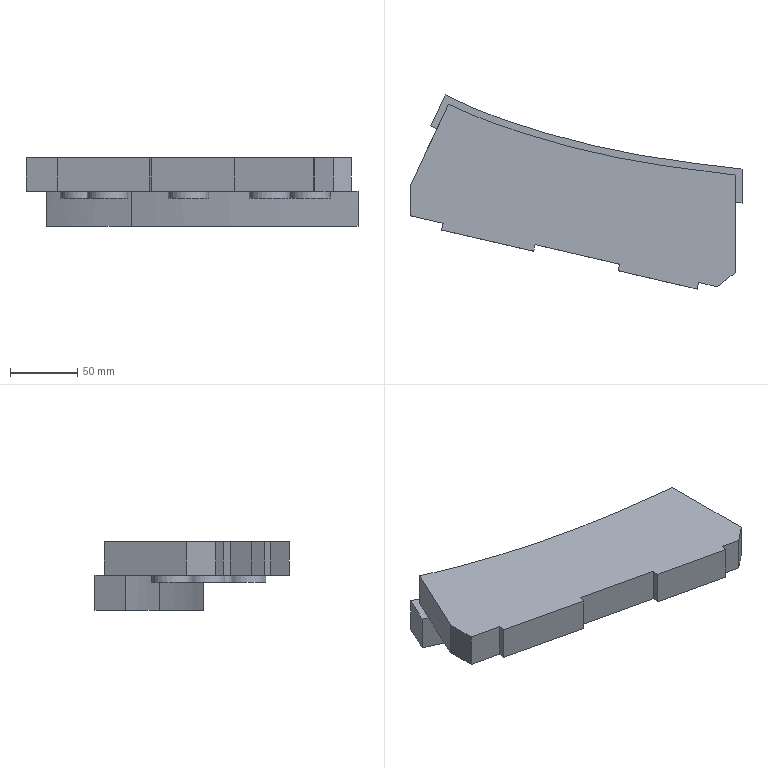Part | NX | features solid 2 | 1 solid | 35 faces | box 246.107 x 143.832 x 51 mm | volume 655442 mm3 | plane 25 | spline 5 | cylinder 5 | commonest cylinder face diameters 30 x5
STEP:
#1=CARTESIAN_POINT('',(-485.611,-295.558,20.));
#2=VERTEX_POINT('',#1);
#3=CARTESIAN_POINT('',(-470.611,-295.558,20.));
#4=DIRECTION('',(0.,0.,-1.));
#5=DIRECTION('',(-1.,0.,0.));
#6=AXIS2_PLACEMENT_3D('',#3,#4,#5);
#7=CIRCLE('',#6,15.);
#8=EDGE_CURVE('',#2,#2,#7,.T.);
#9=ORIENTED_EDGE('',*,*,#8,.F.);
#10=EDGE_LOOP('',(#9));
#11=FACE_BOUND('',#10,.T.);
#12=CARTESIAN_POINT('',(-625.611,-240.558,20.));
#13=VERTEX_POINT('',#12);
#14=CARTESIAN_POINT('',(-610.611,-240.558,20.));
#15=DIRECTION('',(0.,0.,-1.));
#16=DIRECTION('',(-1.,0.,0.));
#17=AXIS2_PLACEMENT_3D('',#14,#15,#16);
#18=CIRCLE('',#17,15.);
#19=EDGE_CURVE('',#13,#13,#18,.T.);
#20=ORIENTED_EDGE('',*,*,#19,.F.);
#21=EDGE_LOOP('',(#20));
#22=FACE_BOUND('',#21,.T.);
#23=CARTESIAN_POINT('',(-410.,-315.453,20.));
#24=VERTEX_POINT('',#23);
#25=CARTESIAN_POINT('',(-410.,-263.355,20.));
#26=VERTEX_POINT('',#25);
#27=CARTESIAN_POINT('',(-410.,-330.218,20.));
#28=DIRECTION('',(0.,-1.,0.));
#29=VECTOR('',#28,1000.);
#30=LINE('',#27,#29);
#31=EDGE_CURVE('',#24,#26,#30,.F.);
#32=ORIENTED_EDGE('',*,*,#31,.F.);
#33=CARTESIAN_POINT('',(-423.262,-326.002,20.));
#34=VERTEX_POINT('',#33);
#35=CARTESIAN_POINT('',(-426.375,-328.478,20.));
#36=DIRECTION('',(-0.7826,-0.6225,0.));
#37=VECTOR('',#36,1000.);
#38=LINE('',#35,#37);
#39=EDGE_CURVE('',#24,#34,#38,.T.);
#40=ORIENTED_EDGE('',*,*,#39,.T.);
#41=CARTESIAN_POINT('',(-437.198,-322.785,20.));
#42=VERTEX_POINT('',#41);
#43=CARTESIAN_POINT('',(-647.681,-274.191,20.));
#44=DIRECTION('',(-0.9744,0.225,0.));
#45=VECTOR('',#44,1000.);
#46=LINE('',#43,#45);
#47=EDGE_CURVE('',#42,#34,#46,.F.);
#48=ORIENTED_EDGE('',*,*,#47,.F.);
#49=CARTESIAN_POINT('',(-438.323,-327.657,20.));
#50=VERTEX_POINT('',#49);
#51=CARTESIAN_POINT('',(-418.412,-241.415,20.));
#52=DIRECTION('',(0.225,0.9744,0.));
#53=VECTOR('',#52,1000.);
#54=LINE('',#51,#53);
#55=EDGE_CURVE('',#42,#50,#54,.F.);
#56=ORIENTED_EDGE('',*,*,#55,.T.);
#57=CARTESIAN_POINT('',(-496.785,-314.16,20.));
#58=VERTEX_POINT('',#57);
#59=CARTESIAN_POINT('',(-360.373,-345.653,20.));
#60=DIRECTION('',(0.9744,-0.225,0.));
#61=VECTOR('',#60,1000.);
#62=LINE('',#59,#61);
#63=EDGE_CURVE('',#58,#50,#62,.T.);
#64=ORIENTED_EDGE('',*,*,#63,.F.);
#65=CARTESIAN_POINT('',(-495.66,-309.288,20.));
#66=VERTEX_POINT('',#65);
#67=CARTESIAN_POINT('',(-476.874,-227.918,20.));
#68=DIRECTION('',(0.225,0.9744,0.));
#69=VECTOR('',#68,1000.);
#70=LINE('',#67,#69);
#71=EDGE_CURVE('',#66,#58,#70,.F.);
#72=ORIENTED_EDGE('',*,*,#71,.F.);
#73=CARTESIAN_POINT('',(-558.405,-294.802,20.));
#74=VERTEX_POINT('',#73);
#75=CARTESIAN_POINT('',(-647.681,-274.191,20.));
#76=DIRECTION('',(-0.9744,0.225,0.));
#77=VECTOR('',#76,1000.);
#78=LINE('',#75,#77);
#79=EDGE_CURVE('',#74,#66,#78,.F.);
#80=ORIENTED_EDGE('',*,*,#79,.F.);
#81=CARTESIAN_POINT('',(-559.529,-299.674,20.));
#82=VERTEX_POINT('',#81);
#83=CARTESIAN_POINT('',(-539.619,-213.432,20.));
#84=DIRECTION('',(0.225,0.9744,0.));
#85=VECTOR('',#84,1000.);
#86=LINE('',#83,#85);
#87=EDGE_CURVE('',#74,#82,#86,.F.);
#88=ORIENTED_EDGE('',*,*,#87,.T.);
#89=CARTESIAN_POINT('',(-627.735,-283.927,20.));
#90=VERTEX_POINT('',#89);
#91=CARTESIAN_POINT('',(-598.504,-290.676,20.));
#92=DIRECTION('',(0.9744,-0.225,0.));
#93=VECTOR('',#92,1000.);
#94=LINE('',#91,#93);
#95=EDGE_CURVE('',#90,#82,#94,.T.);
#96=ORIENTED_EDGE('',*,*,#95,.F.);
#97=CARTESIAN_POINT('',(-626.611,-279.056,20.));
#98=VERTEX_POINT('',#97);
#99=CARTESIAN_POINT('',(-607.825,-197.685,20.));
#100=DIRECTION('',(0.225,0.9744,0.));
#101=VECTOR('',#100,1000.);
#102=LINE('',#99,#101);
#103=EDGE_CURVE('',#98,#90,#102,.F.);
#104=ORIENTED_EDGE('',*,*,#103,.F.);
#105=CARTESIAN_POINT('',(-651.107,-273.4,20.));
#106=VERTEX_POINT('',#105);
#107=CARTESIAN_POINT('',(-647.681,-274.191,20.));
#108=DIRECTION('',(-0.9744,0.225,0.));
#109=VECTOR('',#108,1000.);
#110=LINE('',#107,#109);
#111=EDGE_CURVE('',#106,#98,#110,.F.);
#112=ORIENTED_EDGE('',*,*,#111,.F.);
#113=CARTESIAN_POINT('',(-651.107,-251.643,20.));
#114=VERTEX_POINT('',#113);
#115=CARTESIAN_POINT('',(-651.107,-207.42,20.));
#116=DIRECTION('',(0.,1.,0.));
#117=VECTOR('',#116,1000.);
#118=LINE('',#115,#117);
#119=EDGE_CURVE('',#114,#106,#118,.F.);
#120=ORIENTED_EDGE('',*,*,#119,.F.);
#121=CARTESIAN_POINT('',(-631.107,-208.753,20.));
#122=VERTEX_POINT('',#121);
#123=CARTESIAN_POINT('',(-622.584,-190.474,20.));
#124=DIRECTION('',(0.4226,0.9063,0.));
#125=VECTOR('',#124,1000.);
#126=LINE('',#123,#125);
#127=EDGE_CURVE('',#122,#114,#126,.F.);
#128=ORIENTED_EDGE('',*,*,#127,.F.);
#129=CARTESIAN_POINT('',(-572.969,-231.328,20.));
#130=VERTEX_POINT('',#129);
#131=CARTESIAN_POINT('',(-572.969,-231.328,20.));
#132=CARTESIAN_POINT('',(-592.888,-225.076,20.));
#133=CARTESIAN_POINT('',(-612.439,-217.955,20.));
#134=CARTESIAN_POINT('',(-631.107,-208.753,20.));
#135=B_SPLINE_CURVE_WITH_KNOTS('',3,(#131,#132,#133,#134),.UNSPECIFIED.,.F.,.F.,(4,4),(0.5429,0.6055),.UNSPECIFIED.);
#136=EDGE_CURVE('',#130,#122,#135,.T.);
#137=ORIENTED_EDGE('',*,*,#136,.F.);
#138=CARTESIAN_POINT('',(-572.969,-231.328,20.));
#139=VERTEX_POINT('',#138);
#140=CARTESIAN_POINT('',(-600.393,-321.029,20.));
#141=DIRECTION('',(-0.2924,-0.9563,0.));
#142=VECTOR('',#141,1000.);
#143=LINE('',#140,#142);
#144=EDGE_CURVE('',#130,#139,#143,.F.);
#145=ORIENTED_EDGE('',*,*,#144,.T.);
#146=CARTESIAN_POINT('',(-410.,-263.355,20.));
#147=CARTESIAN_POINT('',(-423.782,-261.77,20.));
#148=CARTESIAN_POINT('',(-451.325,-258.441,20.));
#149=CARTESIAN_POINT('',(-492.449,-252.102,20.));
#150=CARTESIAN_POINT('',(-533.139,-243.268,20.));
#151=CARTESIAN_POINT('',(-559.734,-235.479,20.));
#152=CARTESIAN_POINT('',(-572.969,-231.328,20.));
#153=B_SPLINE_CURVE_WITH_KNOTS('',3,(#146,#147,#148,#149,#150,#151,#152),.UNSPECIFIED.,.F.,.F.,(4,1,1,1,4),(1.31,1.352,1.393,1.435,1.476),.UNSPECIFIED.);
#154=EDGE_CURVE('',#26,#139,#153,.T.);
#155=ORIENTED_EDGE('',*,*,#154,.F.);
#156=EDGE_LOOP('',(#32,#40,#48,#56,#64,#72,#80,#88,#96,#104,#112,#120,#128,#137,#145,#155));
#157=FACE_BOUND('',#156,.T.);
#158=CARTESIAN_POINT('',(-605.611,-265.558,20.));
#159=VERTEX_POINT('',#158);
#160=CARTESIAN_POINT('',(-590.611,-265.558,20.));
#161=DIRECTION('',(0.,0.,-1.));
#162=DIRECTION('',(-1.,0.,0.));
#163=AXIS2_PLACEMENT_3D('',#160,#161,#162);
#164=CIRCLE('',#163,15.);
#165=EDGE_CURVE('',#159,#159,#164,.T.);
#166=ORIENTED_EDGE('',*,*,#165,.F.);
#167=EDGE_LOOP('',(#166));
#168=FACE_BOUND('',#167,.T.);
#169=CARTESIAN_POINT('',(-455.611,-280.558,20.));
#170=VERTEX_POINT('',#169);
#171=CARTESIAN_POINT('',(-440.611,-280.558,20.));
#172=DIRECTION('',(0.,0.,-1.));
#173=DIRECTION('',(-1.,0.,0.));
#174=AXIS2_PLACEMENT_3D('',#171,#172,#173);
#175=CIRCLE('',#174,15.);
#176=EDGE_CURVE('',#170,#170,#175,.T.);
#177=ORIENTED_EDGE('',*,*,#176,.F.);
#178=EDGE_LOOP('',(#177));
#179=FACE_BOUND('',#178,.T.);
#180=CARTESIAN_POINT('',(-545.611,-270.558,20.));
#181=VERTEX_POINT('',#180);
#182=CARTESIAN_POINT('',(-530.611,-270.558,20.));
#183=DIRECTION('',(0.,0.,-1.));
#184=DIRECTION('',(-1.,0.,0.));
#185=AXIS2_PLACEMENT_3D('',#182,#183,#184);
#186=CIRCLE('',#185,15.);
#187=EDGE_CURVE('',#181,#181,#186,.T.);
#188=ORIENTED_EDGE('',*,*,#187,.F.);
#189=EDGE_LOOP('',(#188));
#190=FACE_BOUND('',#189,.T.);
#191=CARTESIAN_POINT('',(-565.659,-207.42,20.));
#192=DIRECTION('',(0.,0.,-1.));
#193=DIRECTION('',(-1.,0.,0.));
#194=AXIS2_PLACEMENT_3D('',#191,#192,#193);
#195=PLANE('',#194);
#196=ADVANCED_FACE('',(#11,#22,#157,#168,#179,#190),#195,.T.);
#197=CARTESIAN_POINT('',(-437.198,-322.785,45.));
#198=VERTEX_POINT('',#197);
#199=CARTESIAN_POINT('',(-423.262,-326.002,45.));
#200=VERTEX_POINT('',#199);
#201=CARTESIAN_POINT('',(-647.681,-274.191,45.));
#202=DIRECTION('',(0.9744,-0.225,0.));
#203=VECTOR('',#202,1000.);
#204=LINE('',#201,#203);
#205=EDGE_CURVE('',#198,#200,#204,.T.);
#206=ORIENTED_EDGE('',*,*,#205,.T.);
#207=CARTESIAN_POINT('',(-410.,-315.453,45.));
#208=VERTEX_POINT('',#207);
#209=CARTESIAN_POINT('',(-891.318,-698.311,45.));
#210=DIRECTION('',(-0.7826,-0.6225,0.));
#211=VECTOR('',#210,1000.);
#212=LINE('',#209,#211);
#213=EDGE_CURVE('',#200,#208,#212,.F.);
#214=ORIENTED_EDGE('',*,*,#213,.T.);
#215=CARTESIAN_POINT('',(-410.,-243.222,45.));
#216=VERTEX_POINT('',#215);
#217=CARTESIAN_POINT('',(-410.,-330.218,45.));
#218=DIRECTION('',(0.,1.,0.));
#219=VECTOR('',#218,1000.);
#220=LINE('',#217,#219);
#221=EDGE_CURVE('',#208,#216,#220,.T.);
#222=ORIENTED_EDGE('',*,*,#221,.T.);
#223=CARTESIAN_POINT('',(-567.121,-212.202,45.));
#224=VERTEX_POINT('',#223);
#225=CARTESIAN_POINT('',(-410.,-243.222,45.));
#226=CARTESIAN_POINT('',(-423.299,-241.685,45.));
#227=CARTESIAN_POINT('',(-449.879,-238.442,45.));
#228=CARTESIAN_POINT('',(-489.484,-232.294,45.));
#229=CARTESIAN_POINT('',(-528.605,-223.762,45.));
#230=CARTESIAN_POINT('',(-554.325,-216.217,45.));
#231=CARTESIAN_POINT('',(-567.121,-212.202,45.));
#232=B_SPLINE_CURVE_WITH_KNOTS('',3,(#225,#226,#227,#228,#229,#230,#231),.UNSPECIFIED.,.F.,.F.,(4,1,1,1,4),(0.1347,0.1748,0.2149,0.2551,0.2952),.UNSPECIFIED.);
#233=EDGE_CURVE('',#216,#224,#232,.T.);
#234=ORIENTED_EDGE('',*,*,#233,.T.);
#235=CARTESIAN_POINT('',(-622.653,-190.623,45.));
#236=VERTEX_POINT('',#235);
#237=CARTESIAN_POINT('',(-567.121,-212.202,45.));
#238=CARTESIAN_POINT('',(-586.224,-206.206,45.));
#239=CARTESIAN_POINT('',(-604.924,-199.397,45.));
#240=CARTESIAN_POINT('',(-622.653,-190.623,45.));
#241=B_SPLINE_CURVE_WITH_KNOTS('',3,(#237,#238,#239,#240),.UNSPECIFIED.,.F.,.F.,(4,4),(0.,0.05934),.UNSPECIFIED.);
#242=EDGE_CURVE('',#224,#236,#241,.T.);
#243=ORIENTED_EDGE('',*,*,#242,.T.);
#244=CARTESIAN_POINT('',(-651.107,-251.643,45.));
#245=VERTEX_POINT('',#244);
#246=CARTESIAN_POINT('',(-622.584,-190.474,45.));
#247=DIRECTION('',(0.4226,0.9063,0.));
#248=VECTOR('',#247,1000.);
#249=LINE('',#246,#248);
#250=EDGE_CURVE('',#236,#245,#249,.F.);
#251=ORIENTED_EDGE('',*,*,#250,.T.);
#252=CARTESIAN_POINT('',(-651.107,-273.4,45.));
#253=VERTEX_POINT('',#252);
#254=CARTESIAN_POINT('',(-651.107,-664.302,45.));
#255=DIRECTION('',(0.,-1.,0.));
#256=VECTOR('',#255,1000.);
#257=LINE('',#254,#256);
#258=EDGE_CURVE('',#245,#253,#257,.T.);
#259=ORIENTED_EDGE('',*,*,#258,.T.);
#260=CARTESIAN_POINT('',(-626.611,-279.056,45.));
#261=VERTEX_POINT('',#260);
#262=CARTESIAN_POINT('',(-647.681,-274.191,45.));
#263=DIRECTION('',(0.9744,-0.225,0.));
#264=VECTOR('',#263,1000.);
#265=LINE('',#262,#264);
#266=EDGE_CURVE('',#253,#261,#265,.T.);
#267=ORIENTED_EDGE('',*,*,#266,.T.);
#268=CARTESIAN_POINT('',(-627.735,-283.927,45.));
#269=VERTEX_POINT('',#268);
#270=CARTESIAN_POINT('',(-725.815,-708.757,45.));
#271=DIRECTION('',(-0.225,-0.9744,0.));
#272=VECTOR('',#271,1000.);
#273=LINE('',#270,#272);
#274=EDGE_CURVE('',#261,#269,#273,.T.);
#275=ORIENTED_EDGE('',*,*,#274,.T.);
#276=CARTESIAN_POINT('',(-559.529,-299.674,45.));
#277=VERTEX_POINT('',#276);
#278=CARTESIAN_POINT('',(-598.504,-290.676,45.));
#279=DIRECTION('',(0.9744,-0.225,0.));
#280=VECTOR('',#279,1000.);
#281=LINE('',#278,#280);
#282=EDGE_CURVE('',#269,#277,#281,.T.);
#283=ORIENTED_EDGE('',*,*,#282,.T.);
#284=CARTESIAN_POINT('',(-558.405,-294.802,45.));
#285=VERTEX_POINT('',#284);
#286=CARTESIAN_POINT('',(-657.609,-724.504,45.));
#287=DIRECTION('',(-0.225,-0.9744,0.));
#288=VECTOR('',#287,1000.);
#289=LINE('',#286,#288);
#290=EDGE_CURVE('',#285,#277,#289,.T.);
#291=ORIENTED_EDGE('',*,*,#290,.F.);
#292=CARTESIAN_POINT('',(-495.66,-309.288,45.));
#293=VERTEX_POINT('',#292);
#294=CARTESIAN_POINT('',(-647.681,-274.191,45.));
#295=DIRECTION('',(0.9744,-0.225,0.));
#296=VECTOR('',#295,1000.);
#297=LINE('',#294,#296);
#298=EDGE_CURVE('',#285,#293,#297,.T.);
#299=ORIENTED_EDGE('',*,*,#298,.T.);
#300=CARTESIAN_POINT('',(-496.785,-314.16,45.));
#301=VERTEX_POINT('',#300);
#302=CARTESIAN_POINT('',(-594.865,-738.989,45.));
#303=DIRECTION('',(-0.225,-0.9744,0.));
#304=VECTOR('',#303,1000.);
#305=LINE('',#302,#304);
#306=EDGE_CURVE('',#293,#301,#305,.T.);
#307=ORIENTED_EDGE('',*,*,#306,.T.);
#308=CARTESIAN_POINT('',(-438.323,-327.657,45.));
#309=VERTEX_POINT('',#308);
#310=CARTESIAN_POINT('',(-360.373,-345.653,45.));
#311=DIRECTION('',(0.9744,-0.225,0.));
#312=VECTOR('',#311,1000.);
#313=LINE('',#310,#312);
#314=EDGE_CURVE('',#301,#309,#313,.T.);
#315=ORIENTED_EDGE('',*,*,#314,.T.);
#316=CARTESIAN_POINT('',(-536.402,-752.486,45.));
#317=DIRECTION('',(-0.225,-0.9744,0.));
#318=VECTOR('',#317,1000.);
#319=LINE('',#316,#318);
#320=EDGE_CURVE('',#198,#309,#319,.T.);
#321=ORIENTED_EDGE('',*,*,#320,.F.);
#322=EDGE_LOOP('',(#206,#214,#222,#234,#243,#251,#259,#267,#275,#283,#291,#299,#307,#315,#321));
#323=FACE_BOUND('',#322,.T.);
#324=CARTESIAN_POINT('',(-918.37,-664.302,45.));
#325=DIRECTION('',(0.,0.,1.));
#326=DIRECTION('',(1.,0.,0.));
#327=AXIS2_PLACEMENT_3D('',#324,#325,#326);
#328=PLANE('',#327);
#329=ADVANCED_FACE('',(#323),#328,.T.);
#330=CARTESIAN_POINT('',(-651.107,-273.4,70.));
#331=DIRECTION('',(0.,0.,1.));
#332=VECTOR('',#331,1000.);
#333=LINE('',#330,#332);
#334=EDGE_CURVE('',#106,#253,#333,.T.);
#335=ORIENTED_EDGE('',*,*,#334,.F.);
#336=ORIENTED_EDGE('',*,*,#111,.T.);
#337=CARTESIAN_POINT('',(-626.611,-279.056,45.));
#338=DIRECTION('',(0.,0.,-1.));
#339=VECTOR('',#338,1000.);
#340=LINE('',#337,#339);
#341=EDGE_CURVE('',#261,#98,#340,.T.);
#342=ORIENTED_EDGE('',*,*,#341,.F.);
#343=ORIENTED_EDGE('',*,*,#266,.F.);
#344=EDGE_LOOP('',(#335,#336,#342,#343));
#345=FACE_BOUND('',#344,.T.);
#346=CARTESIAN_POINT('',(-647.681,-274.191,70.));
#347=DIRECTION('',(0.225,0.9744,0.));
#348=DIRECTION('',(-0.9744,0.225,0.));
#349=AXIS2_PLACEMENT_3D('',#346,#347,#348);
#350=PLANE('',#349);
#351=ADVANCED_FACE('',(#345),#350,.F.);
#352=CARTESIAN_POINT('',(-651.107,-251.643,45.));
#353=DIRECTION('',(0.,0.,-1.));
#354=VECTOR('',#353,1000.);
#355=LINE('',#352,#354);
#356=EDGE_CURVE('',#245,#114,#355,.T.);
#357=ORIENTED_EDGE('',*,*,#356,.F.);
#358=ORIENTED_EDGE('',*,*,#250,.F.);
#359=CARTESIAN_POINT('',(-622.653,-190.623,20.));
#360=VERTEX_POINT('',#359);
#361=CARTESIAN_POINT('',(-622.653,-190.623,32.5));
#362=DIRECTION('',(0.,0.,-1.));
#363=VECTOR('',#362,1000.);
#364=LINE('',#361,#363);
#365=EDGE_CURVE('',#360,#236,#364,.F.);
#366=ORIENTED_EDGE('',*,*,#365,.F.);
#367=CARTESIAN_POINT('',(-622.584,-190.474,20.));
#368=DIRECTION('',(0.4226,0.9063,0.));
#369=VECTOR('',#368,1000.);
#370=LINE('',#367,#369);
#371=EDGE_CURVE('',#360,#122,#370,.F.);
#372=ORIENTED_EDGE('',*,*,#371,.T.);
#373=ORIENTED_EDGE('',*,*,#127,.T.);
#374=EDGE_LOOP('',(#357,#358,#366,#372,#373));
#375=FACE_BOUND('',#374,.T.);
#376=CARTESIAN_POINT('',(-622.584,-190.474,45.));
#377=DIRECTION('',(0.9063,-0.4226,0.));
#378=DIRECTION('',(0.4226,0.9063,0.));
#379=AXIS2_PLACEMENT_3D('',#376,#377,#378);
#380=PLANE('',#379);
#381=ADVANCED_FACE('',(#375),#380,.F.);
#382=CARTESIAN_POINT('',(-625.,-183.825,-6.));
#383=VERTEX_POINT('',#382);
#384=CARTESIAN_POINT('',(-635.575,-206.502,-6.));
#385=VERTEX_POINT('',#384);
#386=CARTESIAN_POINT('',(-861.431,-690.853,-6.));
#387=DIRECTION('',(-0.4226,-0.9063,0.));
#388=VECTOR('',#387,1000.);
#389=LINE('',#386,#388);
#390=EDGE_CURVE('',#383,#385,#389,.T.);
#391=ORIENTED_EDGE('',*,*,#390,.F.);
#392=CARTESIAN_POINT('',(-405.,-238.764,-6.));
#393=VERTEX_POINT('',#392);
#394=CARTESIAN_POINT('',(-625.,-183.825,-6.));
#395=CARTESIAN_POINT('',(-616.501,-188.248,-6.));
#396=CARTESIAN_POINT('',(-599.149,-196.032,-6.));
#397=CARTESIAN_POINT('',(-572.385,-205.497,-6.));
#398=CARTESIAN_POINT('',(-545.206,-213.724,-6.));
#399=CARTESIAN_POINT('',(-517.745,-221.08,-6.));
#400=CARTESIAN_POINT('',(-489.761,-226.95,-6.));
#401=CARTESIAN_POINT('',(-452.233,-233.165,-6.));
#402=CARTESIAN_POINT('',(-423.904,-236.602,-6.));
#403=CARTESIAN_POINT('',(-405.,-238.764,-6.));
#404=B_SPLINE_CURVE_WITH_KNOTS('',3,(#394,#395,#396,#397,#398,#399,#400,#401,#402,#403),.UNSPECIFIED.,.F.,.F.,(4,1,1,1,1,1,1,4),(1.776,1.803,1.83,1.857,1.884,1.911,1.938,1.992),.UNSPECIFIED.);
#405=EDGE_CURVE('',#393,#383,#404,.F.);
#406=ORIENTED_EDGE('',*,*,#405,.F.);
#407=CARTESIAN_POINT('',(-405.,-263.926,-6.));
#408=VERTEX_POINT('',#407);
#409=CARTESIAN_POINT('',(-405.,-1052.635,-6.));
#410=DIRECTION('',(0.,1.,0.));
#411=VECTOR('',#410,1000.);
#412=LINE('',#409,#411);
#413=EDGE_CURVE('',#408,#393,#412,.T.);
#414=ORIENTED_EDGE('',*,*,#413,.F.);
#415=CARTESIAN_POINT('',(-572.969,-231.328,-6.));
#416=VERTEX_POINT('',#415);
#417=CARTESIAN_POINT('',(-405.,-263.926,-6.));
#418=CARTESIAN_POINT('',(-419.214,-262.309,-6.));
#419=CARTESIAN_POINT('',(-447.641,-258.943,-6.));
#420=CARTESIAN_POINT('',(-490.009,-252.558,-6.));
#421=CARTESIAN_POINT('',(-531.843,-243.634,-6.));
#422=CARTESIAN_POINT('',(-559.299,-235.615,-6.));
#423=CARTESIAN_POINT('',(-572.969,-231.328,-6.));
#424=B_SPLINE_CURVE_WITH_KNOTS('',3,(#417,#418,#419,#420,#421,#422,#423),.UNSPECIFIED.,.F.,.F.,(4,1,1,1,4),(0.1254,0.1683,0.2112,0.2541,0.297),.UNSPECIFIED.);
#425=EDGE_CURVE('',#408,#416,#424,.T.);
#426=ORIENTED_EDGE('',*,*,#425,.T.);
#427=CARTESIAN_POINT('',(-572.969,-231.328,-6.));
#428=VERTEX_POINT('',#427);
#429=CARTESIAN_POINT('',(-971.893,-1536.153,-6.));
#430=DIRECTION('',(0.2924,0.9563,0.));
#431=VECTOR('',#430,1000.);
#432=LINE('',#429,#431);
#433=EDGE_CURVE('',#428,#416,#432,.T.);
#434=ORIENTED_EDGE('',*,*,#433,.F.);
#435=CARTESIAN_POINT('',(-572.969,-231.328,-6.));
#436=CARTESIAN_POINT('',(-594.513,-224.566,-6.));
#437=CARTESIAN_POINT('',(-615.605,-216.793,-6.));
#438=CARTESIAN_POINT('',(-635.575,-206.502,-6.));
#439=B_SPLINE_CURVE_WITH_KNOTS('',3,(#435,#436,#437,#438),.UNSPECIFIED.,.F.,.F.,(4,4),(0.,0.06729),.UNSPECIFIED.);
#440=EDGE_CURVE('',#428,#385,#439,.T.);
#441=ORIENTED_EDGE('',*,*,#440,.T.);
#442=EDGE_LOOP('',(#391,#406,#414,#426,#434,#441));
#443=FACE_BOUND('',#442,.T.);
#444=CARTESIAN_POINT('',(-918.37,-664.302,-6.));
#445=DIRECTION('',(0.,0.,1.));
#446=DIRECTION('',(1.,0.,0.));
#447=AXIS2_PLACEMENT_3D('',#444,#445,#446);
#448=PLANE('',#447);
#449=ADVANCED_FACE('',(#443),#448,.F.);
#450=CARTESIAN_POINT('',(-625.,-183.825,20.));
#451=VERTEX_POINT('',#450);
#452=CARTESIAN_POINT('',(-625.,-183.825,7.));
#453=DIRECTION('',(0.,0.,-1.));
#454=VECTOR('',#453,1000.);
#455=LINE('',#452,#454);
#456=EDGE_CURVE('',#451,#383,#455,.T.);
#457=ORIENTED_EDGE('',*,*,#456,.F.);
#458=CARTESIAN_POINT('',(-405.,-238.764,20.));
#459=VERTEX_POINT('',#458);
#460=CARTESIAN_POINT('',(-625.,-183.825,20.));
#461=CARTESIAN_POINT('',(-616.51,-188.243,20.));
#462=CARTESIAN_POINT('',(-599.168,-196.025,20.));
#463=CARTESIAN_POINT('',(-572.395,-205.494,20.));
#464=CARTESIAN_POINT('',(-545.198,-213.727,20.));
#465=CARTESIAN_POINT('',(-517.694,-221.092,20.));
#466=CARTESIAN_POINT('',(-489.704,-226.961,20.));
#467=CARTESIAN_POINT('',(-452.21,-233.167,20.));
#468=CARTESIAN_POINT('',(-423.894,-236.603,20.));
#469=CARTESIAN_POINT('',(-405.,-238.764,20.));
#470=B_SPLINE_CURVE_WITH_KNOTS('',3,(#460,#461,#462,#463,#464,#465,#466,#467,#468,#469),.UNSPECIFIED.,.F.,.F.,(4,1,1,1,1,1,1,4),(1.736,1.763,1.79,1.817,1.844,1.871,1.898,1.952),.UNSPECIFIED.);
#471=EDGE_CURVE('',#459,#451,#470,.F.);
#472=ORIENTED_EDGE('',*,*,#471,.F.);
#473=CARTESIAN_POINT('',(-405.,-238.764,7.));
#474=DIRECTION('',(0.,0.,-1.));
#475=VECTOR('',#474,1000.);
#476=LINE('',#473,#475);
#477=EDGE_CURVE('',#393,#459,#476,.F.);
#478=ORIENTED_EDGE('',*,*,#477,.F.);
#479=ORIENTED_EDGE('',*,*,#405,.T.);
#480=EDGE_LOOP('',(#457,#472,#478,#479));
#481=FACE_BOUND('',#480,.T.);
#482=CARTESIAN_POINT('',(-405.,-238.764,20.));
#483=CARTESIAN_POINT('',(-405.,-238.764,-6.));
#484=CARTESIAN_POINT('',(-423.871,-236.605,20.));
#485=CARTESIAN_POINT('',(-423.871,-236.605,-6.));
#486=CARTESIAN_POINT('',(-452.167,-233.174,20.));
#487=CARTESIAN_POINT('',(-452.167,-233.174,-6.));
#488=CARTESIAN_POINT('',(-489.652,-226.969,20.));
#489=CARTESIAN_POINT('',(-489.652,-226.969,-6.));
#490=CARTESIAN_POINT('',(-517.544,-221.127,20.));
#491=CARTESIAN_POINT('',(-517.544,-221.127,-6.));
#492=CARTESIAN_POINT('',(-545.076,-213.764,20.));
#493=CARTESIAN_POINT('',(-545.076,-213.764,-6.));
#494=CARTESIAN_POINT('',(-572.351,-205.509,20.));
#495=CARTESIAN_POINT('',(-572.351,-205.509,-6.));
#496=CARTESIAN_POINT('',(-599.224,-196.006,20.));
#497=CARTESIAN_POINT('',(-599.224,-196.006,-6.));
#498=CARTESIAN_POINT('',(-616.576,-188.209,20.));
#499=CARTESIAN_POINT('',(-616.576,-188.209,-6.));
#500=CARTESIAN_POINT('',(-625.,-183.825,20.));
#501=CARTESIAN_POINT('',(-625.,-183.825,-6.));
#502=B_SPLINE_SURFACE_WITH_KNOTS('',3,1,((#482,#483),(#484,#485),(#486,#487),(#488,#489),(#490,#491),(#492,#493),(#494,#495),(#496,#497),(#498,#499),(#500,#501)),.SURF_OF_LINEAR_EXTRUSION.,.F.,.F.,.F.,(4,1,1,1,1,1,1,4),(2,2),(0.5985,0.6471,0.6714,0.6957,0.7201,0.7444,0.7687,0.793),(0.,1.),.UNSPECIFIED.);
#503=ADVANCED_FACE('',(#481),#502,.F.);
#504=ORIENTED_EDGE('',*,*,#471,.T.);
#505=CARTESIAN_POINT('',(-635.575,-206.502,20.));
#506=VERTEX_POINT('',#505);
#507=CARTESIAN_POINT('',(-623.439,-180.477,20.));
#508=DIRECTION('',(-0.4226,-0.9063,0.));
#509=VECTOR('',#508,1000.);
#510=LINE('',#507,#509);
#511=EDGE_CURVE('',#506,#451,#510,.F.);
#512=ORIENTED_EDGE('',*,*,#511,.F.);
#513=CARTESIAN_POINT('',(-631.107,-208.753,20.));
#514=CARTESIAN_POINT('',(-632.6,-208.018,20.));
#515=CARTESIAN_POINT('',(-634.089,-207.268,20.));
#516=CARTESIAN_POINT('',(-635.575,-206.502,20.));
#517=B_SPLINE_CURVE_WITH_KNOTS('',3,(#513,#514,#515,#516),.UNSPECIFIED.,.F.,.F.,(4,4),(0.1938,0.2089),.UNSPECIFIED.);
#518=EDGE_CURVE('',#122,#506,#517,.T.);
#519=ORIENTED_EDGE('',*,*,#518,.F.);
#520=ORIENTED_EDGE('',*,*,#371,.F.);
#521=CARTESIAN_POINT('',(-567.121,-212.202,20.));
#522=VERTEX_POINT('',#521);
#523=CARTESIAN_POINT('',(-567.121,-212.202,20.));
#524=CARTESIAN_POINT('',(-586.127,-206.236,20.));
#525=CARTESIAN_POINT('',(-604.937,-199.391,20.));
#526=CARTESIAN_POINT('',(-622.653,-190.623,20.));
#527=B_SPLINE_CURVE_WITH_KNOTS('',3,(#523,#524,#525,#526),.UNSPECIFIED.,.F.,.F.,(4,4),(0.6706,0.7303),.UNSPECIFIED.);
#528=EDGE_CURVE('',#522,#360,#527,.T.);
#529=ORIENTED_EDGE('',*,*,#528,.F.);
#530=CARTESIAN_POINT('',(-410.,-243.222,20.));
#531=VERTEX_POINT('',#530);
#532=CARTESIAN_POINT('',(-410.,-243.222,20.));
#533=CARTESIAN_POINT('',(-423.289,-241.686,20.));
#534=CARTESIAN_POINT('',(-449.843,-238.447,20.));
#535=CARTESIAN_POINT('',(-489.497,-232.294,20.));
#536=CARTESIAN_POINT('',(-528.717,-223.733,20.));
#537=CARTESIAN_POINT('',(-554.359,-216.207,20.));
#538=CARTESIAN_POINT('',(-567.121,-212.202,20.));
#539=B_SPLINE_CURVE_WITH_KNOTS('',3,(#532,#533,#534,#535,#536,#537,#538),.UNSPECIFIED.,.F.,.F.,(4,1,1,1,4),(1.314,1.354,1.395,1.435,1.475),.UNSPECIFIED.);
#540=EDGE_CURVE('',#531,#522,#539,.T.);
#541=ORIENTED_EDGE('',*,*,#540,.F.);
#542=CARTESIAN_POINT('',(-410.,-330.218,20.));
#543=DIRECTION('',(0.,-1.,0.));
#544=VECTOR('',#543,1000.);
#545=LINE('',#542,#544);
#546=EDGE_CURVE('',#26,#531,#545,.F.);
#547=ORIENTED_EDGE('',*,*,#546,.F.);
#548=CARTESIAN_POINT('',(-405.,-263.926,20.));
#549=VERTEX_POINT('',#548);
#550=CARTESIAN_POINT('',(-405.,-263.926,20.));
#551=CARTESIAN_POINT('',(-406.667,-263.737,20.));
#552=CARTESIAN_POINT('',(-408.333,-263.546,20.));
#553=CARTESIAN_POINT('',(-410.,-263.355,20.));
#554=B_SPLINE_CURVE_WITH_KNOTS('',3,(#550,#551,#552,#553),.UNSPECIFIED.,.F.,.F.,(4,4),(1.305,1.31),.UNSPECIFIED.);
#555=EDGE_CURVE('',#549,#26,#554,.T.);
#556=ORIENTED_EDGE('',*,*,#555,.F.);
#557=CARTESIAN_POINT('',(-405.,-401.561,20.));
#558=DIRECTION('',(0.,1.,0.));
#559=VECTOR('',#558,1000.);
#560=LINE('',#557,#559);
#561=EDGE_CURVE('',#459,#549,#560,.F.);
#562=ORIENTED_EDGE('',*,*,#561,.F.);
#563=EDGE_LOOP('',(#504,#512,#519,#520,#529,#541,#547,#556,#562));
#564=FACE_BOUND('',#563,.T.);
#565=CARTESIAN_POINT('',(-565.659,-207.42,20.));
#566=DIRECTION('',(0.,0.,1.));
#567=DIRECTION('',(1.,0.,0.));
#568=AXIS2_PLACEMENT_3D('',#565,#566,#567);
#569=PLANE('',#568);
#570=ADVANCED_FACE('',(#564),#569,.T.);
#571=ORIENTED_EDGE('',*,*,#528,.T.);
#572=ORIENTED_EDGE('',*,*,#365,.T.);
#573=ORIENTED_EDGE('',*,*,#242,.F.);
#574=CARTESIAN_POINT('',(-567.121,-212.202,32.5));
#575=DIRECTION('',(0.,0.,-1.));
#576=VECTOR('',#575,1000.);
#577=LINE('',#574,#576);
#578=EDGE_CURVE('',#224,#522,#577,.T.);
#579=ORIENTED_EDGE('',*,*,#578,.T.);
#580=EDGE_LOOP('',(#571,#572,#573,#579));
#581=FACE_BOUND('',#580,.T.);
#582=CARTESIAN_POINT('',(-567.121,-212.202,45.));
#583=CARTESIAN_POINT('',(-567.121,-212.202,20.));
#584=CARTESIAN_POINT('',(-571.801,-210.733,45.));
#585=CARTESIAN_POINT('',(-571.801,-210.733,20.));
#586=CARTESIAN_POINT('',(-581.265,-207.651,45.));
#587=CARTESIAN_POINT('',(-581.265,-207.651,20.));
#588=CARTESIAN_POINT('',(-599.914,-200.932,45.));
#589=CARTESIAN_POINT('',(-599.914,-200.932,20.));
#590=CARTESIAN_POINT('',(-613.692,-195.058,45.));
#591=CARTESIAN_POINT('',(-613.692,-195.058,20.));
#592=CARTESIAN_POINT('',(-622.653,-190.623,45.));
#593=CARTESIAN_POINT('',(-622.653,-190.623,20.));
#594=B_SPLINE_SURFACE_WITH_KNOTS('',3,1,((#582,#583),(#584,#585),(#586,#587),(#588,#589),(#590,#591),(#592,#593)),.SURF_OF_LINEAR_EXTRUSION.,.F.,.F.,.F.,(4,1,1,4),(2,2),(-0.0001232,0.04872,0.09756,0.1952),(0.,1.),.UNSPECIFIED.);
#595=ADVANCED_FACE('',(#581),#594,.F.);
#596=CARTESIAN_POINT('',(-635.575,-206.502,7.));
#597=DIRECTION('',(0.,0.,1.));
#598=VECTOR('',#597,1000.);
#599=LINE('',#596,#598);
#600=EDGE_CURVE('',#385,#506,#599,.T.);
#601=ORIENTED_EDGE('',*,*,#600,.F.);
#602=ORIENTED_EDGE('',*,*,#440,.F.);
#603=CARTESIAN_POINT('',(-572.969,-231.328,9.5));
#604=DIRECTION('',(0.,0.,1.));
#605=VECTOR('',#604,1000.);
#606=LINE('',#603,#605);
#607=EDGE_CURVE('',#428,#130,#606,.T.);
#608=ORIENTED_EDGE('',*,*,#607,.T.);
#609=ORIENTED_EDGE('',*,*,#136,.T.);
#610=ORIENTED_EDGE('',*,*,#518,.T.);
#611=EDGE_LOOP('',(#601,#602,#608,#609,#610));
#612=FACE_BOUND('',#611,.T.);
#613=CARTESIAN_POINT('',(-572.969,-231.328,-6.));
#614=CARTESIAN_POINT('',(-572.969,-231.328,20.));
#615=CARTESIAN_POINT('',(-574.224,-230.934,-6.));
#616=CARTESIAN_POINT('',(-574.224,-230.934,20.));
#617=CARTESIAN_POINT('',(-576.883,-230.093,-6.));
#618=CARTESIAN_POINT('',(-576.883,-230.093,20.));
#619=CARTESIAN_POINT('',(-582.081,-228.409,-6.));
#620=CARTESIAN_POINT('',(-582.081,-228.409,20.));
#621=CARTESIAN_POINT('',(-591.26,-225.327,-6.));
#622=CARTESIAN_POINT('',(-591.26,-225.327,20.));
#623=CARTESIAN_POINT('',(-604.35,-220.565,-6.));
#624=CARTESIAN_POINT('',(-604.35,-220.565,20.));
#625=CARTESIAN_POINT('',(-620.044,-214.092,-6.));
#626=CARTESIAN_POINT('',(-620.044,-214.092,20.));
#627=CARTESIAN_POINT('',(-630.427,-209.155,-6.));
#628=CARTESIAN_POINT('',(-630.427,-209.155,20.));
#629=CARTESIAN_POINT('',(-635.575,-206.502,-6.));
#630=CARTESIAN_POINT('',(-635.575,-206.502,20.));
#631=B_SPLINE_SURFACE_WITH_KNOTS('',3,1,((#613,#614),(#615,#616),(#617,#618),(#619,#620),(#621,#622),(#623,#624),(#625,#626),(#627,#628),(#629,#630)),.SURF_OF_LINEAR_EXTRUSION.,.F.,.F.,.F.,(4,1,1,1,1,1,4),(2,2),(-0.0006161,0.01248,0.02558,0.05177,0.1042,0.1566,0.2089),(0.,1.),.UNSPECIFIED.);
#632=ADVANCED_FACE('',(#612),#631,.F.);
#633=ORIENTED_EDGE('',*,*,#144,.F.);
#634=ORIENTED_EDGE('',*,*,#607,.F.);
#635=ORIENTED_EDGE('',*,*,#433,.T.);
#636=CARTESIAN_POINT('',(-572.969,-231.328,9.5));
#637=DIRECTION('',(0.,0.,1.));
#638=VECTOR('',#637,1000.);
#639=LINE('',#636,#638);
#640=EDGE_CURVE('',#139,#416,#639,.F.);
#641=ORIENTED_EDGE('',*,*,#640,.F.);
#642=EDGE_LOOP('',(#633,#634,#635,#641));
#643=FACE_BOUND('',#642,.T.);
#644=CARTESIAN_POINT('',(-971.893,-1536.153,70.));
#645=DIRECTION('',(-0.9563,0.2924,0.));
#646=DIRECTION('',(-0.2924,-0.9563,0.));
#647=AXIS2_PLACEMENT_3D('',#644,#645,#646);
#648=PLANE('',#647);
#649=ADVANCED_FACE('',(#643),#648,.F.);
#650=ORIENTED_EDGE('',*,*,#47,.T.);
#651=CARTESIAN_POINT('',(-423.262,-326.002,70.));
#652=DIRECTION('',(0.,0.,-1.));
#653=VECTOR('',#652,1000.);
#654=LINE('',#651,#653);
#655=EDGE_CURVE('',#34,#200,#654,.F.);
#656=ORIENTED_EDGE('',*,*,#655,.T.);
#657=ORIENTED_EDGE('',*,*,#205,.F.);
#658=CARTESIAN_POINT('',(-437.198,-322.785,45.));
#659=DIRECTION('',(0.,0.,-1.));
#660=VECTOR('',#659,1000.);
#661=LINE('',#658,#660);
#662=EDGE_CURVE('',#198,#42,#661,.T.);
#663=ORIENTED_EDGE('',*,*,#662,.T.);
#664=EDGE_LOOP('',(#650,#656,#657,#663));
#665=FACE_BOUND('',#664,.T.);
#666=CARTESIAN_POINT('',(-647.681,-274.191,70.));
#667=DIRECTION('',(0.225,0.9744,0.));
#668=DIRECTION('',(-0.9744,0.225,0.));
#669=AXIS2_PLACEMENT_3D('',#666,#667,#668);
#670=PLANE('',#669);
#671=ADVANCED_FACE('',(#665),#670,.F.);
#672=ORIENTED_EDGE('',*,*,#233,.F.);
#673=CARTESIAN_POINT('',(-410.,-243.222,32.5));
#674=DIRECTION('',(0.,0.,-1.));
#675=VECTOR('',#674,1000.);
#676=LINE('',#673,#675);
#677=EDGE_CURVE('',#216,#531,#676,.T.);
#678=ORIENTED_EDGE('',*,*,#677,.T.);
#679=ORIENTED_EDGE('',*,*,#540,.T.);
#680=ORIENTED_EDGE('',*,*,#578,.F.);
#681=EDGE_LOOP('',(#672,#678,#679,#680));
#682=FACE_BOUND('',#681,.T.);
#683=CARTESIAN_POINT('',(-410.,-243.222,45.));
#684=CARTESIAN_POINT('',(-410.,-243.222,20.));
#685=CARTESIAN_POINT('',(-423.223,-241.693,45.));
#686=CARTESIAN_POINT('',(-423.223,-241.693,20.));
#687=CARTESIAN_POINT('',(-449.692,-238.468,45.));
#688=CARTESIAN_POINT('',(-449.692,-238.468,20.));
#689=CARTESIAN_POINT('',(-489.327,-232.32,45.));
#690=CARTESIAN_POINT('',(-489.327,-232.32,20.));
#691=CARTESIAN_POINT('',(-522.118,-225.195,45.));
#692=CARTESIAN_POINT('',(-522.118,-225.195,20.));
#693=CARTESIAN_POINT('',(-547.961,-218.055,45.));
#694=CARTESIAN_POINT('',(-547.961,-218.055,20.));
#695=CARTESIAN_POINT('',(-560.734,-214.206,45.));
#696=CARTESIAN_POINT('',(-560.734,-214.206,20.));
#697=CARTESIAN_POINT('',(-567.121,-212.202,45.));
#698=CARTESIAN_POINT('',(-567.121,-212.202,20.));
#699=B_SPLINE_SURFACE_WITH_KNOTS('',3,1,((#683,#684),(#685,#686),(#687,#688),(#689,#690),(#691,#692),(#693,#694),(#695,#696),(#697,#698)),.SURF_OF_LINEAR_EXTRUSION.,.F.,.F.,.F.,(4,1,1,1,1,4),(2,2),(0.4587,0.594,0.7293,0.8646,0.9322,0.9999),(0.,1.),.UNSPECIFIED.);
#700=ADVANCED_FACE('',(#682),#699,.F.);
#701=CARTESIAN_POINT('',(-405.,-263.926,7.));
#702=DIRECTION('',(0.,0.,1.));
#703=VECTOR('',#702,1000.);
#704=LINE('',#701,#703);
#705=EDGE_CURVE('',#549,#408,#704,.F.);
#706=ORIENTED_EDGE('',*,*,#705,.F.);
#707=ORIENTED_EDGE('',*,*,#555,.T.);
#708=ORIENTED_EDGE('',*,*,#154,.T.);
#709=ORIENTED_EDGE('',*,*,#640,.T.);
#710=ORIENTED_EDGE('',*,*,#425,.F.);
#711=EDGE_LOOP('',(#706,#707,#708,#709,#710));
#712=FACE_BOUND('',#711,.T.);
#713=CARTESIAN_POINT('',(-405.,-263.926,-6.));
#714=CARTESIAN_POINT('',(-405.,-263.926,20.));
#715=CARTESIAN_POINT('',(-418.868,-262.349,-6.));
#716=CARTESIAN_POINT('',(-418.868,-262.349,20.));
#717=CARTESIAN_POINT('',(-446.791,-259.053,-6.));
#718=CARTESIAN_POINT('',(-446.791,-259.053,20.));
#719=CARTESIAN_POINT('',(-482.029,-253.767,-6.));
#720=CARTESIAN_POINT('',(-482.029,-253.767,20.));
#721=CARTESIAN_POINT('',(-510.39,-248.239,-6.));
#722=CARTESIAN_POINT('',(-510.39,-248.239,20.));
#723=CARTESIAN_POINT('',(-531.607,-243.291,-6.));
#724=CARTESIAN_POINT('',(-531.607,-243.291,20.));
#725=CARTESIAN_POINT('',(-552.567,-237.556,-6.));
#726=CARTESIAN_POINT('',(-552.567,-237.556,20.));
#727=CARTESIAN_POINT('',(-566.106,-233.48,-6.));
#728=CARTESIAN_POINT('',(-566.106,-233.48,20.));
#729=CARTESIAN_POINT('',(-572.969,-231.328,-6.));
#730=CARTESIAN_POINT('',(-572.969,-231.328,20.));
#731=B_SPLINE_SURFACE_WITH_KNOTS('',3,1,((#713,#714),(#715,#716),(#717,#718),(#719,#720),(#721,#722),(#723,#724),(#725,#726),(#727,#728),(#729,#730)),.SURF_OF_LINEAR_EXTRUSION.,.F.,.F.,.F.,(4,1,1,1,1,1,4),(2,2),(0.4339,0.5753,0.7166,0.7873,0.858,0.9287,0.9994),(0.,1.),.UNSPECIFIED.);
#732=ADVANCED_FACE('',(#712),#731,.F.);
#733=CARTESIAN_POINT('',(-558.405,-294.802,45.));
#734=DIRECTION('',(0.,0.,-1.));
#735=VECTOR('',#734,1000.);
#736=LINE('',#733,#735);
#737=EDGE_CURVE('',#285,#74,#736,.T.);
#738=ORIENTED_EDGE('',*,*,#737,.T.);
#739=ORIENTED_EDGE('',*,*,#79,.T.);
#740=CARTESIAN_POINT('',(-495.66,-309.288,45.));
#741=DIRECTION('',(0.,0.,-1.));
#742=VECTOR('',#741,1000.);
#743=LINE('',#740,#742);
#744=EDGE_CURVE('',#293,#66,#743,.T.);
#745=ORIENTED_EDGE('',*,*,#744,.F.);
#746=ORIENTED_EDGE('',*,*,#298,.F.);
#747=EDGE_LOOP('',(#738,#739,#745,#746));
#748=FACE_BOUND('',#747,.T.);
#749=CARTESIAN_POINT('',(-647.681,-274.191,70.));
#750=DIRECTION('',(0.225,0.9744,0.));
#751=DIRECTION('',(-0.9744,0.225,0.));
#752=AXIS2_PLACEMENT_3D('',#749,#750,#751);
#753=PLANE('',#752);
#754=ADVANCED_FACE('',(#748),#753,.F.);
#755=CARTESIAN_POINT('',(-438.323,-327.657,45.));
#756=DIRECTION('',(0.,0.,-1.));
#757=VECTOR('',#756,1000.);
#758=LINE('',#755,#757);
#759=EDGE_CURVE('',#309,#50,#758,.T.);
#760=ORIENTED_EDGE('',*,*,#759,.T.);
#761=ORIENTED_EDGE('',*,*,#55,.F.);
#762=ORIENTED_EDGE('',*,*,#662,.F.);
#763=ORIENTED_EDGE('',*,*,#320,.T.);
#764=EDGE_LOOP('',(#760,#761,#762,#763));
#765=FACE_BOUND('',#764,.T.);
#766=CARTESIAN_POINT('',(-437.198,-322.785,45.));
#767=DIRECTION('',(-0.9744,0.225,0.));
#768=DIRECTION('',(-0.225,-0.9744,0.));
#769=AXIS2_PLACEMENT_3D('',#766,#767,#768);
#770=PLANE('',#769);
#771=ADVANCED_FACE('',(#765),#770,.F.);
#772=CARTESIAN_POINT('',(-496.785,-314.16,45.));
#773=DIRECTION('',(0.,0.,-1.));
#774=VECTOR('',#773,1000.);
#775=LINE('',#772,#774);
#776=EDGE_CURVE('',#301,#58,#775,.T.);
#777=ORIENTED_EDGE('',*,*,#776,.F.);
#778=ORIENTED_EDGE('',*,*,#306,.F.);
#779=ORIENTED_EDGE('',*,*,#744,.T.);
#780=ORIENTED_EDGE('',*,*,#71,.T.);
#781=EDGE_LOOP('',(#777,#778,#779,#780));
#782=FACE_BOUND('',#781,.T.);
#783=CARTESIAN_POINT('',(-495.66,-309.288,45.));
#784=DIRECTION('',(-0.9744,0.225,0.));
#785=DIRECTION('',(-0.225,-0.9744,0.));
#786=AXIS2_PLACEMENT_3D('',#783,#784,#785);
#787=PLANE('',#786);
#788=ADVANCED_FACE('',(#782),#787,.T.);
#789=ORIENTED_EDGE('',*,*,#759,.F.);
#790=ORIENTED_EDGE('',*,*,#314,.F.);
#791=ORIENTED_EDGE('',*,*,#776,.T.);
#792=ORIENTED_EDGE('',*,*,#63,.T.);
#793=EDGE_LOOP('',(#789,#790,#791,#792));
#794=FACE_BOUND('',#793,.T.);
#795=CARTESIAN_POINT('',(-360.373,-345.653,45.));
#796=DIRECTION('',(-0.225,-0.9744,0.));
#797=DIRECTION('',(0.,0.,-1.));
#798=AXIS2_PLACEMENT_3D('',#795,#796,#797);
#799=PLANE('',#798);
#800=ADVANCED_FACE('',(#794),#799,.T.);
#801=CARTESIAN_POINT('',(-559.529,-299.674,45.));
#802=DIRECTION('',(0.,0.,-1.));
#803=VECTOR('',#802,1000.);
#804=LINE('',#801,#803);
#805=EDGE_CURVE('',#277,#82,#804,.T.);
#806=ORIENTED_EDGE('',*,*,#805,.T.);
#807=ORIENTED_EDGE('',*,*,#87,.F.);
#808=ORIENTED_EDGE('',*,*,#737,.F.);
#809=ORIENTED_EDGE('',*,*,#290,.T.);
#810=EDGE_LOOP('',(#806,#807,#808,#809));
#811=FACE_BOUND('',#810,.T.);
#812=CARTESIAN_POINT('',(-558.405,-294.802,45.));
#813=DIRECTION('',(-0.9744,0.225,0.));
#814=DIRECTION('',(-0.225,-0.9744,0.));
#815=AXIS2_PLACEMENT_3D('',#812,#813,#814);
#816=PLANE('',#815);
#817=ADVANCED_FACE('',(#811),#816,.F.);
#818=CARTESIAN_POINT('',(-627.735,-283.927,45.));
#819=DIRECTION('',(0.,0.,-1.));
#820=VECTOR('',#819,1000.);
#821=LINE('',#818,#820);
#822=EDGE_CURVE('',#269,#90,#821,.T.);
#823=ORIENTED_EDGE('',*,*,#822,.F.);
#824=ORIENTED_EDGE('',*,*,#274,.F.);
#825=ORIENTED_EDGE('',*,*,#341,.T.);
#826=ORIENTED_EDGE('',*,*,#103,.T.);
#827=EDGE_LOOP('',(#823,#824,#825,#826));
#828=FACE_BOUND('',#827,.T.);
#829=CARTESIAN_POINT('',(-626.611,-279.056,45.));
#830=DIRECTION('',(-0.9744,0.225,0.));
#831=DIRECTION('',(-0.225,-0.9744,0.));
#832=AXIS2_PLACEMENT_3D('',#829,#830,#831);
#833=PLANE('',#832);
#834=ADVANCED_FACE('',(#828),#833,.T.);
#835=ORIENTED_EDGE('',*,*,#805,.F.);
#836=ORIENTED_EDGE('',*,*,#282,.F.);
#837=ORIENTED_EDGE('',*,*,#822,.T.);
#838=ORIENTED_EDGE('',*,*,#95,.T.);
#839=EDGE_LOOP('',(#835,#836,#837,#838));
#840=FACE_BOUND('',#839,.T.);
#841=CARTESIAN_POINT('',(-598.504,-290.676,45.));
#842=DIRECTION('',(-0.225,-0.9744,0.));
#843=DIRECTION('',(0.,0.,-1.));
#844=AXIS2_PLACEMENT_3D('',#841,#842,#843);
#845=PLANE('',#844);
#846=ADVANCED_FACE('',(#840),#845,.T.);
#847=ORIENTED_EDGE('',*,*,#561,.T.);
#848=ORIENTED_EDGE('',*,*,#705,.T.);
#849=ORIENTED_EDGE('',*,*,#413,.T.);
#850=ORIENTED_EDGE('',*,*,#477,.T.);
#851=EDGE_LOOP('',(#847,#848,#849,#850));
#852=FACE_BOUND('',#851,.T.);
#853=CARTESIAN_POINT('',(-405.,-560.,0.));
#854=DIRECTION('',(1.,0.,0.));
#855=DIRECTION('',(0.,0.,-1.));
#856=AXIS2_PLACEMENT_3D('',#853,#854,#855);
#857=PLANE('',#856);
#858=ADVANCED_FACE('',(#852),#857,.T.);
#859=ORIENTED_EDGE('',*,*,#221,.F.);
#860=CARTESIAN_POINT('',(-410.,-315.453,70.));
#861=DIRECTION('',(0.,0.,1.));
#862=VECTOR('',#861,1000.);
#863=LINE('',#860,#862);
#864=EDGE_CURVE('',#208,#24,#863,.F.);
#865=ORIENTED_EDGE('',*,*,#864,.T.);
#866=ORIENTED_EDGE('',*,*,#31,.T.);
#867=ORIENTED_EDGE('',*,*,#546,.T.);
#868=ORIENTED_EDGE('',*,*,#677,.F.);
#869=EDGE_LOOP('',(#859,#865,#866,#867,#868));
#870=FACE_BOUND('',#869,.T.);
#871=CARTESIAN_POINT('',(-410.,-330.218,45.));
#872=DIRECTION('',(-1.,0.,0.));
#873=DIRECTION('',(0.,0.,1.));
#874=AXIS2_PLACEMENT_3D('',#871,#872,#873);
#875=PLANE('',#874);
#876=ADVANCED_FACE('',(#870),#875,.F.);
#877=ORIENTED_EDGE('',*,*,#600,.T.);
#878=ORIENTED_EDGE('',*,*,#511,.T.);
#879=ORIENTED_EDGE('',*,*,#456,.T.);
#880=ORIENTED_EDGE('',*,*,#390,.T.);
#881=EDGE_LOOP('',(#877,#878,#879,#880));
#882=FACE_BOUND('',#881,.T.);
#883=CARTESIAN_POINT('',(-783.978,-524.755,0.));
#884=DIRECTION('',(-0.9063,0.4226,0.));
#885=DIRECTION('',(-0.4226,-0.9063,0.));
#886=AXIS2_PLACEMENT_3D('',#883,#884,#885);
#887=PLANE('',#886);
#888=ADVANCED_FACE('',(#882),#887,.T.);
#889=ORIENTED_EDGE('',*,*,#119,.T.);
#890=ORIENTED_EDGE('',*,*,#334,.T.);
#891=ORIENTED_EDGE('',*,*,#258,.F.);
#892=ORIENTED_EDGE('',*,*,#356,.T.);
#893=EDGE_LOOP('',(#889,#890,#891,#892));
#894=FACE_BOUND('',#893,.T.);
#895=CARTESIAN_POINT('',(-651.107,-361.69,20.));
#896=DIRECTION('',(-1.,0.,0.));
#897=DIRECTION('',(0.,-1.,0.));
#898=AXIS2_PLACEMENT_3D('',#895,#896,#897);
#899=PLANE('',#898);
#900=ADVANCED_FACE('',(#894),#899,.T.);
#901=ORIENTED_EDGE('',*,*,#39,.F.);
#902=ORIENTED_EDGE('',*,*,#864,.F.);
#903=ORIENTED_EDGE('',*,*,#213,.F.);
#904=ORIENTED_EDGE('',*,*,#655,.F.);
#905=EDGE_LOOP('',(#901,#902,#903,#904));
#906=FACE_BOUND('',#905,.T.);
#907=CARTESIAN_POINT('',(-426.375,-328.478,70.));
#908=DIRECTION('',(-0.6225,0.7826,0.));
#909=DIRECTION('',(-0.7826,-0.6225,0.));
#910=AXIS2_PLACEMENT_3D('',#907,#908,#909);
#911=PLANE('',#910);
#912=ADVANCED_FACE('',(#906),#911,.F.);
#913=CARTESIAN_POINT('',(-575.611,-265.558,15.));
#914=VERTEX_POINT('',#913);
#915=CARTESIAN_POINT('',(-590.611,-265.558,15.));
#916=DIRECTION('',(0.,0.,1.));
#917=DIRECTION('',(1.,0.,0.));
#918=AXIS2_PLACEMENT_3D('',#915,#916,#917);
#919=CIRCLE('',#918,15.);
#920=EDGE_CURVE('',#914,#914,#919,.T.);
#921=ORIENTED_EDGE('',*,*,#920,.T.);
#922=EDGE_LOOP('',(#921));
#923=FACE_BOUND('',#922,.T.);
#924=ORIENTED_EDGE('',*,*,#165,.T.);
#925=EDGE_LOOP('',(#924));
#926=FACE_BOUND('',#925,.T.);
#927=CARTESIAN_POINT('',(-590.611,-265.558,25.));
#928=DIRECTION('',(0.,0.,-1.));
#929=DIRECTION('',(-1.,0.,0.));
#930=AXIS2_PLACEMENT_3D('',#927,#928,#929);
#931=CYLINDRICAL_SURFACE('',#930,15.);
#932=ADVANCED_FACE('',(#923,#926),#931,.T.);
#933=ORIENTED_EDGE('',*,*,#920,.F.);
#934=EDGE_LOOP('',(#933));
#935=FACE_BOUND('',#934,.T.);
#936=CARTESIAN_POINT('',(-590.611,-265.558,15.));
#937=DIRECTION('',(0.,0.,1.));
#938=DIRECTION('',(1.,0.,0.));
#939=AXIS2_PLACEMENT_3D('',#936,#937,#938);
#940=PLANE('',#939);
#941=ADVANCED_FACE('',(#935),#940,.F.);
#942=CARTESIAN_POINT('',(-595.611,-240.558,15.));
#943=VERTEX_POINT('',#942);
#944=CARTESIAN_POINT('',(-610.611,-240.558,15.));
#945=DIRECTION('',(0.,0.,1.));
#946=DIRECTION('',(1.,0.,0.));
#947=AXIS2_PLACEMENT_3D('',#944,#945,#946);
#948=CIRCLE('',#947,15.);
#949=EDGE_CURVE('',#943,#943,#948,.T.);
#950=ORIENTED_EDGE('',*,*,#949,.T.);
#951=EDGE_LOOP('',(#950));
#952=FACE_BOUND('',#951,.T.);
#953=ORIENTED_EDGE('',*,*,#19,.T.);
#954=EDGE_LOOP('',(#953));
#955=FACE_BOUND('',#954,.T.);
#956=CARTESIAN_POINT('',(-610.611,-240.558,25.));
#957=DIRECTION('',(0.,0.,-1.));
#958=DIRECTION('',(-1.,0.,0.));
#959=AXIS2_PLACEMENT_3D('',#956,#957,#958);
#960=CYLINDRICAL_SURFACE('',#959,15.);
#961=ADVANCED_FACE('',(#952,#955),#960,.T.);
#962=ORIENTED_EDGE('',*,*,#949,.F.);
#963=EDGE_LOOP('',(#962));
#964=FACE_BOUND('',#963,.T.);
#965=CARTESIAN_POINT('',(-610.611,-240.558,15.));
#966=DIRECTION('',(0.,0.,1.));
#967=DIRECTION('',(1.,0.,0.));
#968=AXIS2_PLACEMENT_3D('',#965,#966,#967);
#969=PLANE('',#968);
#970=ADVANCED_FACE('',(#964),#969,.F.);
#971=CARTESIAN_POINT('',(-425.611,-280.558,15.));
#972=VERTEX_POINT('',#971);
#973=CARTESIAN_POINT('',(-440.611,-280.558,15.));
#974=DIRECTION('',(0.,0.,1.));
#975=DIRECTION('',(1.,0.,0.));
#976=AXIS2_PLACEMENT_3D('',#973,#974,#975);
#977=CIRCLE('',#976,15.);
#978=EDGE_CURVE('',#972,#972,#977,.T.);
#979=ORIENTED_EDGE('',*,*,#978,.T.);
#980=EDGE_LOOP('',(#979));
#981=FACE_BOUND('',#980,.T.);
#982=ORIENTED_EDGE('',*,*,#176,.T.);
#983=EDGE_LOOP('',(#982));
#984=FACE_BOUND('',#983,.T.);
#985=CARTESIAN_POINT('',(-440.611,-280.558,25.));
#986=DIRECTION('',(0.,0.,-1.));
#987=DIRECTION('',(-1.,0.,0.));
#988=AXIS2_PLACEMENT_3D('',#985,#986,#987);
#989=CYLINDRICAL_SURFACE('',#988,15.);
#990=ADVANCED_FACE('',(#981,#984),#989,.T.);
#991=ORIENTED_EDGE('',*,*,#978,.F.);
#992=EDGE_LOOP('',(#991));
#993=FACE_BOUND('',#992,.T.);
#994=CARTESIAN_POINT('',(-440.611,-280.558,15.));
#995=DIRECTION('',(0.,0.,1.));
#996=DIRECTION('',(1.,0.,0.));
#997=AXIS2_PLACEMENT_3D('',#994,#995,#996);
#998=PLANE('',#997);
#999=ADVANCED_FACE('',(#993),#998,.F.);
#1000=CARTESIAN_POINT('',(-455.611,-295.558,15.));
#1001=VERTEX_POINT('',#1000);
#1002=CARTESIAN_POINT('',(-470.611,-295.558,15.));
#1003=DIRECTION('',(0.,0.,1.));
#1004=DIRECTION('',(1.,0.,0.));
#1005=AXIS2_PLACEMENT_3D('',#1002,#1003,#1004);
#1006=CIRCLE('',#1005,15.);
#1007=EDGE_CURVE('',#1001,#1001,#1006,.T.);
#1008=ORIENTED_EDGE('',*,*,#1007,.T.);
#1009=EDGE_LOOP('',(#1008));
#1010=FACE_BOUND('',#1009,.T.);
#1011=ORIENTED_EDGE('',*,*,#8,.T.);
#1012=EDGE_LOOP('',(#1011));
#1013=FACE_BOUND('',#1012,.T.);
#1014=CARTESIAN_POINT('',(-470.611,-295.558,25.));
#1015=DIRECTION('',(0.,0.,-1.));
#1016=DIRECTION('',(-1.,0.,0.));
#1017=AXIS2_PLACEMENT_3D('',#1014,#1015,#1016);
#1018=CYLINDRICAL_SURFACE('',#1017,15.);
#1019=ADVANCED_FACE('',(#1010,#1013),#1018,.T.);
#1020=ORIENTED_EDGE('',*,*,#1007,.F.);
#1021=EDGE_LOOP('',(#1020));
#1022=FACE_BOUND('',#1021,.T.);
#1023=CARTESIAN_POINT('',(-470.611,-295.558,15.));
#1024=DIRECTION('',(0.,0.,1.));
#1025=DIRECTION('',(1.,0.,0.));
#1026=AXIS2_PLACEMENT_3D('',#1023,#1024,#1025);
#1027=PLANE('',#1026);
#1028=ADVANCED_FACE('',(#1022),#1027,.F.);
#1029=CARTESIAN_POINT('',(-515.611,-270.558,15.));
#1030=VERTEX_POINT('',#1029);
#1031=CARTESIAN_POINT('',(-530.611,-270.558,15.));
#1032=DIRECTION('',(0.,0.,1.));
#1033=DIRECTION('',(1.,0.,0.));
#1034=AXIS2_PLACEMENT_3D('',#1031,#1032,#1033);
#1035=CIRCLE('',#1034,15.);
#1036=EDGE_CURVE('',#1030,#1030,#1035,.T.);
#1037=ORIENTED_EDGE('',*,*,#1036,.T.);
#1038=EDGE_LOOP('',(#1037));
#1039=FACE_BOUND('',#1038,.T.);
#1040=ORIENTED_EDGE('',*,*,#187,.T.);
#1041=EDGE_LOOP('',(#1040));
#1042=FACE_BOUND('',#1041,.T.);
#1043=CARTESIAN_POINT('',(-530.611,-270.558,25.));
#1044=DIRECTION('',(0.,0.,-1.));
#1045=DIRECTION('',(-1.,0.,0.));
#1046=AXIS2_PLACEMENT_3D('',#1043,#1044,#1045);
#1047=CYLINDRICAL_SURFACE('',#1046,15.);
#1048=ADVANCED_FACE('',(#1039,#1042),#1047,.T.);
#1049=ORIENTED_EDGE('',*,*,#1036,.F.);
#1050=EDGE_LOOP('',(#1049));
#1051=FACE_BOUND('',#1050,.T.);
#1052=CARTESIAN_POINT('',(-530.611,-270.558,15.));
#1053=DIRECTION('',(0.,0.,1.));
#1054=DIRECTION('',(1.,0.,0.));
#1055=AXIS2_PLACEMENT_3D('',#1052,#1053,#1054);
#1056=PLANE('',#1055);
#1057=ADVANCED_FACE('',(#1051),#1056,.F.);
#1058=CLOSED_SHELL('',(#196,#329,#351,#381,#449,#503,#570,#595,#632,#649,#671,#700,#732,#754,#771,#788,#800,#817,#834,#846,#858,#876,#888,#900,#912,#932,#941,#961,#970,#990,#999,#1019,#1028,#1048,#1057));
#1059=MANIFOLD_SOLID_BREP('',#1058);
#1060=(LENGTH_UNIT()NAMED_UNIT(*)SI_UNIT(.MILLI.,.METRE.));
#1061=UNCERTAINTY_MEASURE_WITH_UNIT(LENGTH_MEASURE(0.0508),#1060,'','');
#1062=(NAMED_UNIT(*)PLANE_ANGLE_UNIT()SI_UNIT($,.RADIAN.));
#1063=(NAMED_UNIT(*)SI_UNIT($,.STERADIAN.)SOLID_ANGLE_UNIT());
#1064=(GEOMETRIC_REPRESENTATION_CONTEXT(3)GLOBAL_UNCERTAINTY_ASSIGNED_CONTEXT((#1061))GLOBAL_UNIT_ASSIGNED_CONTEXT((#1060,#1062,#1063))REPRESENTATION_CONTEXT('',''));
#1065=ADVANCED_BREP_SHAPE_REPRESENTATION('',(#1059),#1064);